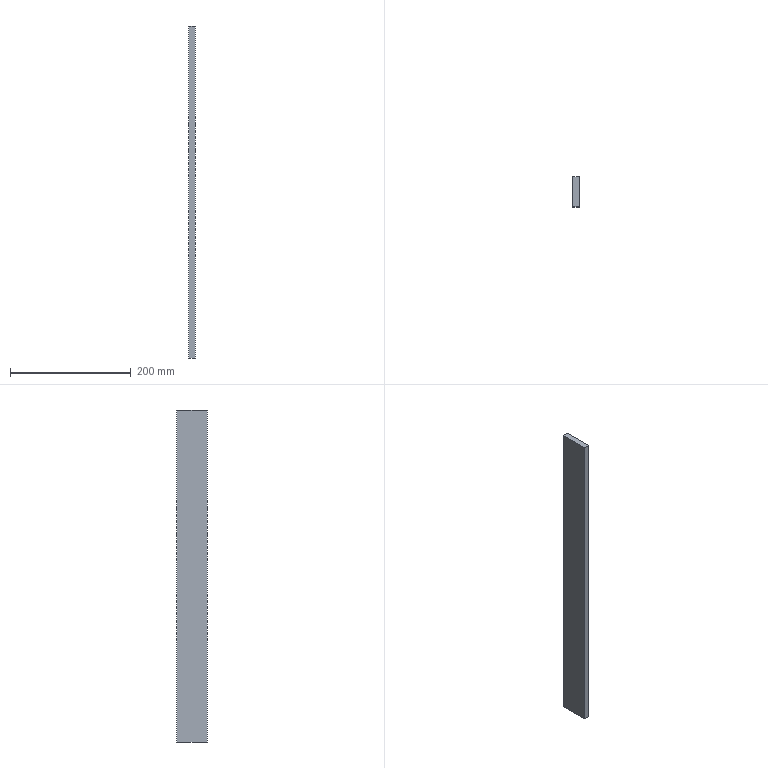Part | NX | features solid 2 | 1 solid | 6 faces | box 10 x 50 x 550 mm | volume 275000 mm3 | plane 6
STEP:
#1=CARTESIAN_POINT('',(1160.,490.,80.));
#2=VERTEX_POINT('',#1);
#3=CARTESIAN_POINT('',(1160.,440.,80.));
#4=VERTEX_POINT('',#3);
#5=CARTESIAN_POINT('',(1160.,490.,80.));
#6=DIRECTION('',(0.,-1.,0.));
#7=VECTOR('',#6,1000.);
#8=LINE('',#5,#7);
#9=EDGE_CURVE('',#2,#4,#8,.T.);
#10=ORIENTED_EDGE('',*,*,#9,.F.);
#11=CARTESIAN_POINT('',(1160.,490.,-470.));
#12=VERTEX_POINT('',#11);
#13=CARTESIAN_POINT('',(1160.,490.,70.));
#14=DIRECTION('',(0.,0.,-1.));
#15=VECTOR('',#14,1000.);
#16=LINE('',#13,#15);
#17=EDGE_CURVE('',#2,#12,#16,.T.);
#18=ORIENTED_EDGE('',*,*,#17,.T.);
#19=CARTESIAN_POINT('',(1160.,440.,-470.));
#20=VERTEX_POINT('',#19);
#21=CARTESIAN_POINT('',(1160.,490.,-470.));
#22=DIRECTION('',(0.,-1.,0.));
#23=VECTOR('',#22,1000.);
#24=LINE('',#21,#23);
#25=EDGE_CURVE('',#12,#20,#24,.T.);
#26=ORIENTED_EDGE('',*,*,#25,.T.);
#27=CARTESIAN_POINT('',(1160.,440.,70.));
#28=DIRECTION('',(0.,0.,-1.));
#29=VECTOR('',#28,1000.);
#30=LINE('',#27,#29);
#31=EDGE_CURVE('',#4,#20,#30,.T.);
#32=ORIENTED_EDGE('',*,*,#31,.F.);
#33=EDGE_LOOP('',(#10,#18,#26,#32));
#34=FACE_BOUND('',#33,.T.);
#35=CARTESIAN_POINT('',(1160.,490.,70.));
#36=DIRECTION('',(-1.,0.,0.));
#37=DIRECTION('',(0.,0.,1.));
#38=AXIS2_PLACEMENT_3D('',#35,#36,#37);
#39=PLANE('',#38);
#40=ADVANCED_FACE('',(#34),#39,.T.);
#41=ORIENTED_EDGE('',*,*,#25,.F.);
#42=CARTESIAN_POINT('',(1170.,490.,-470.));
#43=VERTEX_POINT('',#42);
#44=CARTESIAN_POINT('',(1160.,490.,-470.));
#45=DIRECTION('',(1.,0.,0.));
#46=VECTOR('',#45,1000.);
#47=LINE('',#44,#46);
#48=EDGE_CURVE('',#12,#43,#47,.T.);
#49=ORIENTED_EDGE('',*,*,#48,.T.);
#50=CARTESIAN_POINT('',(1170.,440.,-470.));
#51=VERTEX_POINT('',#50);
#52=CARTESIAN_POINT('',(1170.,490.,-470.));
#53=DIRECTION('',(0.,-1.,0.));
#54=VECTOR('',#53,1000.);
#55=LINE('',#52,#54);
#56=EDGE_CURVE('',#43,#51,#55,.T.);
#57=ORIENTED_EDGE('',*,*,#56,.T.);
#58=CARTESIAN_POINT('',(1160.,440.,-470.));
#59=DIRECTION('',(1.,0.,0.));
#60=VECTOR('',#59,1000.);
#61=LINE('',#58,#60);
#62=EDGE_CURVE('',#20,#51,#61,.T.);
#63=ORIENTED_EDGE('',*,*,#62,.F.);
#64=EDGE_LOOP('',(#41,#49,#57,#63));
#65=FACE_BOUND('',#64,.T.);
#66=CARTESIAN_POINT('',(1160.,490.,-470.));
#67=DIRECTION('',(0.,0.,-1.));
#68=DIRECTION('',(-1.,0.,0.));
#69=AXIS2_PLACEMENT_3D('',#66,#67,#68);
#70=PLANE('',#69);
#71=ADVANCED_FACE('',(#65),#70,.T.);
#72=ORIENTED_EDGE('',*,*,#56,.F.);
#73=CARTESIAN_POINT('',(1170.,490.,80.));
#74=VERTEX_POINT('',#73);
#75=CARTESIAN_POINT('',(1170.,490.,70.));
#76=DIRECTION('',(0.,0.,-1.));
#77=VECTOR('',#76,1000.);
#78=LINE('',#75,#77);
#79=EDGE_CURVE('',#74,#43,#78,.T.);
#80=ORIENTED_EDGE('',*,*,#79,.F.);
#81=CARTESIAN_POINT('',(1170.,440.,80.));
#82=VERTEX_POINT('',#81);
#83=CARTESIAN_POINT('',(1170.,490.,80.));
#84=DIRECTION('',(0.,-1.,0.));
#85=VECTOR('',#84,1000.);
#86=LINE('',#83,#85);
#87=EDGE_CURVE('',#74,#82,#86,.T.);
#88=ORIENTED_EDGE('',*,*,#87,.T.);
#89=CARTESIAN_POINT('',(1170.,440.,70.));
#90=DIRECTION('',(0.,0.,-1.));
#91=VECTOR('',#90,1000.);
#92=LINE('',#89,#91);
#93=EDGE_CURVE('',#82,#51,#92,.T.);
#94=ORIENTED_EDGE('',*,*,#93,.T.);
#95=EDGE_LOOP('',(#72,#80,#88,#94));
#96=FACE_BOUND('',#95,.T.);
#97=CARTESIAN_POINT('',(1170.,490.,70.));
#98=DIRECTION('',(-1.,0.,0.));
#99=DIRECTION('',(0.,0.,1.));
#100=AXIS2_PLACEMENT_3D('',#97,#98,#99);
#101=PLANE('',#100);
#102=ADVANCED_FACE('',(#96),#101,.F.);
#103=CARTESIAN_POINT('',(1160.,490.,80.));
#104=DIRECTION('',(1.,0.,0.));
#105=VECTOR('',#104,1000.);
#106=LINE('',#103,#105);
#107=EDGE_CURVE('',#2,#74,#106,.T.);
#108=ORIENTED_EDGE('',*,*,#107,.F.);
#109=ORIENTED_EDGE('',*,*,#9,.T.);
#110=CARTESIAN_POINT('',(1160.,440.,80.));
#111=DIRECTION('',(1.,0.,0.));
#112=VECTOR('',#111,1000.);
#113=LINE('',#110,#112);
#114=EDGE_CURVE('',#4,#82,#113,.T.);
#115=ORIENTED_EDGE('',*,*,#114,.T.);
#116=ORIENTED_EDGE('',*,*,#87,.F.);
#117=EDGE_LOOP('',(#108,#109,#115,#116));
#118=FACE_BOUND('',#117,.T.);
#119=CARTESIAN_POINT('',(1160.,490.,80.));
#120=DIRECTION('',(0.,0.,-1.));
#121=DIRECTION('',(-1.,0.,0.));
#122=AXIS2_PLACEMENT_3D('',#119,#120,#121);
#123=PLANE('',#122);
#124=ADVANCED_FACE('',(#118),#123,.F.);
#125=ORIENTED_EDGE('',*,*,#93,.F.);
#126=ORIENTED_EDGE('',*,*,#114,.F.);
#127=ORIENTED_EDGE('',*,*,#31,.T.);
#128=ORIENTED_EDGE('',*,*,#62,.T.);
#129=EDGE_LOOP('',(#125,#126,#127,#128));
#130=FACE_BOUND('',#129,.T.);
#131=CARTESIAN_POINT('',(1160.,440.,70.));
#132=DIRECTION('',(0.,1.,0.));
#133=DIRECTION('',(0.,0.,-1.));
#134=AXIS2_PLACEMENT_3D('',#131,#132,#133);
#135=PLANE('',#134);
#136=ADVANCED_FACE('',(#130),#135,.F.);
#137=ORIENTED_EDGE('',*,*,#79,.T.);
#138=ORIENTED_EDGE('',*,*,#48,.F.);
#139=ORIENTED_EDGE('',*,*,#17,.F.);
#140=ORIENTED_EDGE('',*,*,#107,.T.);
#141=EDGE_LOOP('',(#137,#138,#139,#140));
#142=FACE_BOUND('',#141,.T.);
#143=CARTESIAN_POINT('',(1160.,490.,70.));
#144=DIRECTION('',(0.,1.,0.));
#145=DIRECTION('',(0.,0.,-1.));
#146=AXIS2_PLACEMENT_3D('',#143,#144,#145);
#147=PLANE('',#146);
#148=ADVANCED_FACE('',(#142),#147,.T.);
#149=CLOSED_SHELL('',(#40,#71,#102,#124,#136,#148));
#150=MANIFOLD_SOLID_BREP('',#149);
#151=(LENGTH_UNIT()NAMED_UNIT(*)SI_UNIT(.MILLI.,.METRE.));
#152=UNCERTAINTY_MEASURE_WITH_UNIT(LENGTH_MEASURE(0.00001),#151,'','');
#153=(NAMED_UNIT(*)PLANE_ANGLE_UNIT()SI_UNIT($,.RADIAN.));
#154=(NAMED_UNIT(*)SI_UNIT($,.STERADIAN.)SOLID_ANGLE_UNIT());
#155=(GEOMETRIC_REPRESENTATION_CONTEXT(3)GLOBAL_UNCERTAINTY_ASSIGNED_CONTEXT((#152))GLOBAL_UNIT_ASSIGNED_CONTEXT((#151,#153,#154))REPRESENTATION_CONTEXT('',''));
#156=ADVANCED_BREP_SHAPE_REPRESENTATION('',(#150),#155);